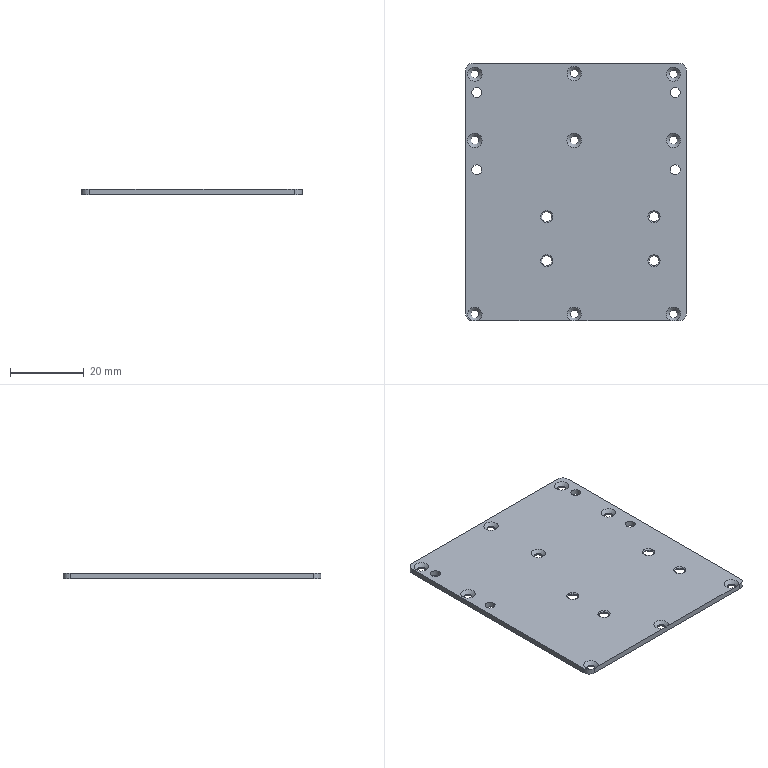Part | STEP file | VSWR protection cover | 1 solid | 53 faces | box 60 x 70.12 x 1.5 mm | volume 6124 mm3 | cone 26 | cylinder 21 | plane 6 | commonest cylinder face diameters 2.2 x9 2.7 x8 4 x4